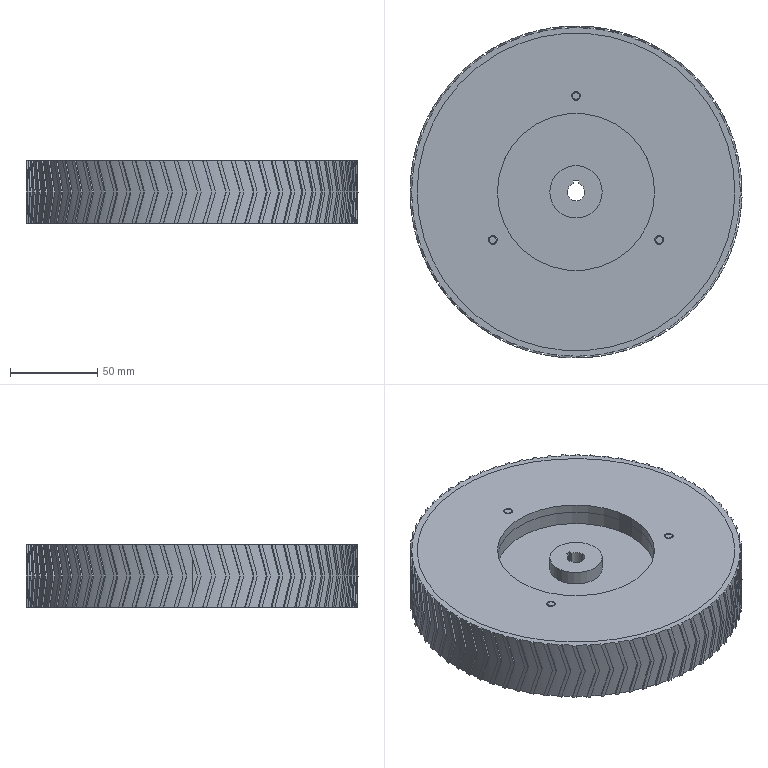Part | SolidWorks | 8 solids | 519 faces | box 190.182 x 190.182 x 36 mm | volume 833820 mm3 | plane 383 | cylinder 124 | cone 12 | commonest cylinder face diameters 188 x73 5 x24 90 x8 182 x6 30 x4 130 x4